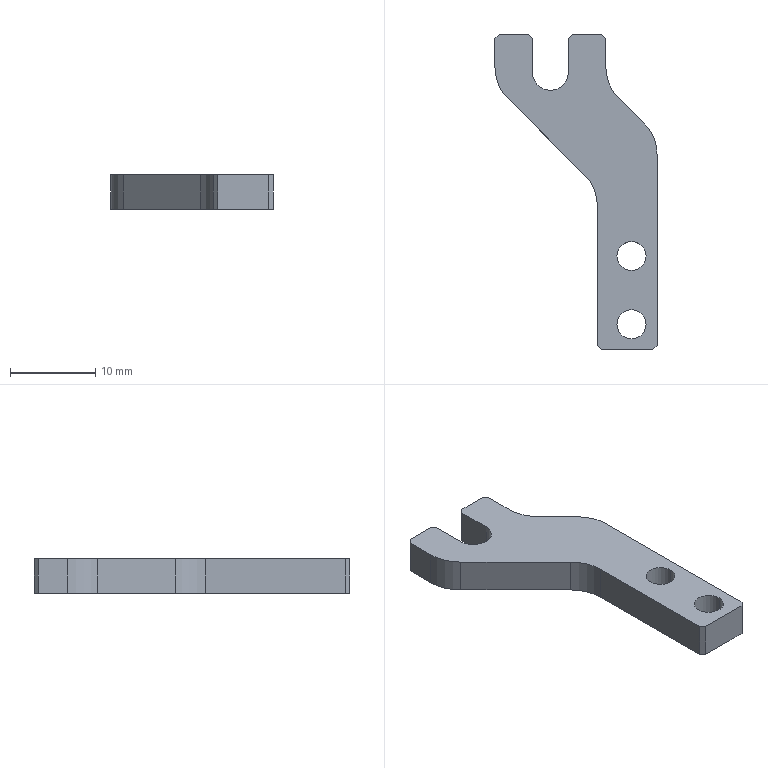Part | STEP file | Stopper bar mounting plate | 1 solid | 28 faces | box 19 x 37 x 4 mm | volume 1217 mm3 | plane 19 | cylinder 9 | commonest cylinder face diameters 3.4 x4 10 x4 4.2 x1